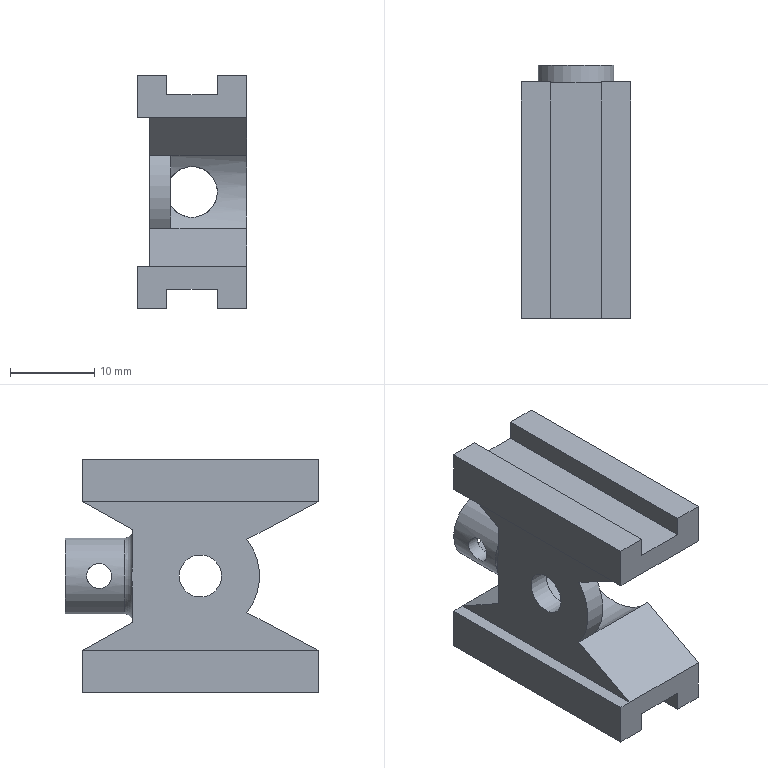Part | STEP file | 2-06.4 | 1 solid | 42 faces | box 13 x 30 x 27.66 mm | volume 5154 mm3 | plane 32 | cylinder 9 | torus 1 | commonest cylinder face diameters 2 x2 3 x2 14 x2 5 x1 6 x1 9 x1